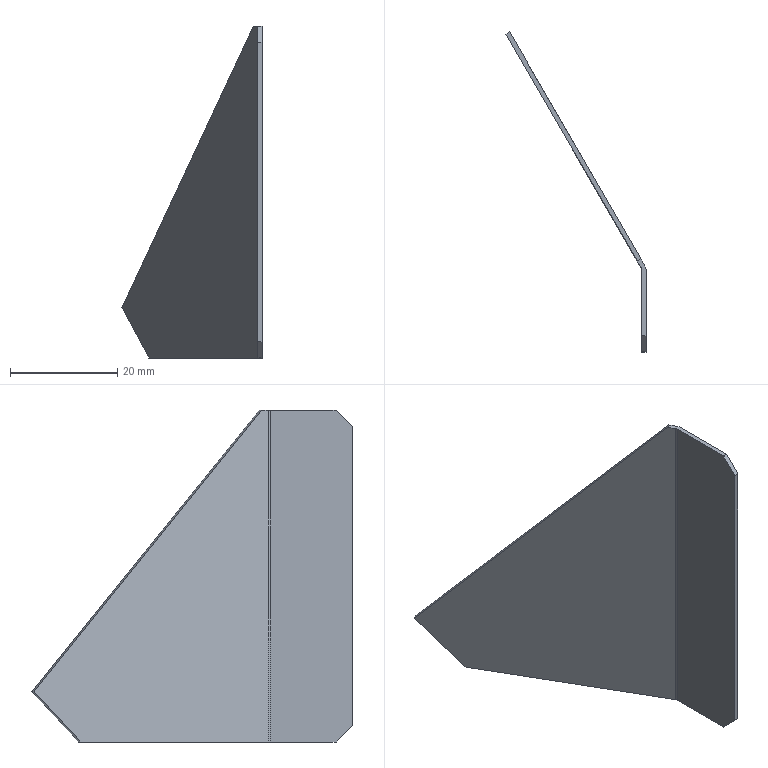Part | SolidWorks | features BaseBody 1 | 1 solid | 13 faces | box 26.168 x 59.793 x 62 mm | volume 2216 mm3 | plane 11 | cylinder 2 | commonest cylinder face diameters 1.473 x1 3.073 x1
STEP:
#1=CARTESIAN_POINT('',(267.101,174.773,-56.848));
#2=VERTEX_POINT('',#1);
#3=CARTESIAN_POINT('',(246.859,209.834,-56.848));
#4=VERTEX_POINT('',#3);
#5=CARTESIAN_POINT('',(256.98,192.304,-56.848));
#6=DIRECTION('',(-0.5,0.866,0.));
#7=VECTOR('',#6,1000.);
#8=LINE('',#5,#7);
#9=EDGE_CURVE('',#2,#4,#8,.T.);
#10=ORIENTED_EDGE('',*,*,#9,.T.);
#11=CARTESIAN_POINT('',(247.552,210.234,-56.848));
#12=VERTEX_POINT('',#11);
#13=CARTESIAN_POINT('',(247.205,210.034,-56.848));
#14=DIRECTION('',(-0.866,-0.5,0.));
#15=VECTOR('',#14,1000.);
#16=LINE('',#13,#15);
#17=EDGE_CURVE('',#12,#4,#16,.T.);
#18=ORIENTED_EDGE('',*,*,#17,.F.);
#19=CARTESIAN_POINT('',(267.794,175.173,-56.848));
#20=VERTEX_POINT('',#19);
#21=CARTESIAN_POINT('',(257.673,192.704,-56.848));
#22=DIRECTION('',(0.5,-0.866,0.));
#23=VECTOR('',#22,1000.);
#24=LINE('',#21,#23);
#25=EDGE_CURVE('',#12,#20,#24,.T.);
#26=ORIENTED_EDGE('',*,*,#25,.T.);
#27=CARTESIAN_POINT('',(268.,174.405,-56.848));
#28=VERTEX_POINT('',#27);
#29=CARTESIAN_POINT('',(266.463,174.405,-56.848));
#30=DIRECTION('',(0.,0.,-1.));
#31=DIRECTION('',(-1.,0.,0.));
#32=AXIS2_PLACEMENT_3D('',#29,#30,#31);
#33=CIRCLE('',#32,1.537);
#34=EDGE_CURVE('',#20,#28,#33,.T.);
#35=ORIENTED_EDGE('',*,*,#34,.T.);
#36=CARTESIAN_POINT('',(268.,162.147,-56.848));
#37=VERTEX_POINT('',#36);
#38=CARTESIAN_POINT('',(268.,166.776,-56.848));
#39=DIRECTION('',(0.,1.,0.));
#40=VECTOR('',#39,1000.);
#41=LINE('',#38,#40);
#42=EDGE_CURVE('',#37,#28,#41,.T.);
#43=ORIENTED_EDGE('',*,*,#42,.F.);
#44=CARTESIAN_POINT('',(267.2,162.147,-56.848));
#45=VERTEX_POINT('',#44);
#46=CARTESIAN_POINT('',(267.6,162.147,-56.848));
#47=DIRECTION('',(-1.,0.,0.));
#48=VECTOR('',#47,1000.);
#49=LINE('',#46,#48);
#50=EDGE_CURVE('',#37,#45,#49,.T.);
#51=ORIENTED_EDGE('',*,*,#50,.T.);
#52=CARTESIAN_POINT('',(267.2,174.405,-56.848));
#53=VERTEX_POINT('',#52);
#54=CARTESIAN_POINT('',(267.2,166.776,-56.848));
#55=DIRECTION('',(0.,1.,0.));
#56=VECTOR('',#55,1000.);
#57=LINE('',#54,#56);
#58=EDGE_CURVE('',#45,#53,#57,.T.);
#59=ORIENTED_EDGE('',*,*,#58,.T.);
#60=CARTESIAN_POINT('',(266.463,174.405,-56.848));
#61=DIRECTION('',(0.,0.,-1.));
#62=DIRECTION('',(-1.,0.,0.));
#63=AXIS2_PLACEMENT_3D('',#60,#61,#62);
#64=CIRCLE('',#63,0.7366);
#65=EDGE_CURVE('',#2,#53,#64,.T.);
#66=ORIENTED_EDGE('',*,*,#65,.F.);
#67=EDGE_LOOP('',(#10,#18,#26,#35,#43,#51,#59,#66));
#68=FACE_OUTER_BOUND('',#67,.T.);
#69=CARTESIAN_POINT('',(267.101,174.773,-56.848));
#70=DIRECTION('',(0.,0.,-1.));
#71=DIRECTION('',(-0.5,0.866,0.));
#72=AXIS2_PLACEMENT_3D('',#69,#70,#71);
#73=PLANE('',#72);
#74=ADVANCED_FACE('',(#68),#73,.T.);
#75=CARTESIAN_POINT('',(266.35,176.075,5.152));
#76=VERTEX_POINT('',#75);
#77=CARTESIAN_POINT('',(267.101,174.773,5.152));
#78=VERTEX_POINT('',#77);
#79=CARTESIAN_POINT('',(254.467,196.657,5.152));
#80=DIRECTION('',(0.5,-0.866,0.));
#81=VECTOR('',#80,1000.);
#82=LINE('',#79,#81);
#83=EDGE_CURVE('',#76,#78,#82,.T.);
#84=ORIENTED_EDGE('',*,*,#83,.F.);
#85=CARTESIAN_POINT('',(241.832,218.54,-47.483));
#86=VERTEX_POINT('',#85);
#87=CARTESIAN_POINT('',(241.832,218.54,-47.483));
#88=DIRECTION('',(0.3408,-0.5903,0.7317));
#89=VECTOR('',#88,1000.);
#90=LINE('',#87,#89);
#91=EDGE_CURVE('',#86,#76,#90,.T.);
#92=ORIENTED_EDGE('',*,*,#91,.F.);
#93=CARTESIAN_POINT('',(246.859,209.834,-56.848));
#94=DIRECTION('',(-0.3658,0.6337,0.6816));
#95=VECTOR('',#94,1000.);
#96=LINE('',#93,#95);
#97=EDGE_CURVE('',#4,#86,#96,.T.);
#98=ORIENTED_EDGE('',*,*,#97,.F.);
#99=ORIENTED_EDGE('',*,*,#9,.F.);
#100=CARTESIAN_POINT('',(267.101,174.773,-25.848));
#101=DIRECTION('',(0.,0.,-1.));
#102=VECTOR('',#101,1000.);
#103=LINE('',#100,#102);
#104=EDGE_CURVE('',#78,#2,#103,.T.);
#105=ORIENTED_EDGE('',*,*,#104,.F.);
#106=EDGE_LOOP('',(#84,#92,#98,#99,#105));
#107=FACE_OUTER_BOUND('',#106,.T.);
#108=CARTESIAN_POINT('',(267.101,174.773,5.152));
#109=DIRECTION('',(0.866,0.5,0.));
#110=DIRECTION('',(0.,0.,-1.));
#111=AXIS2_PLACEMENT_3D('',#108,#109,#110);
#112=PLANE('',#111);
#113=ADVANCED_FACE('',(#107),#112,.F.);
#114=CARTESIAN_POINT('',(242.525,218.94,-47.483));
#115=VERTEX_POINT('',#114);
#116=CARTESIAN_POINT('',(247.552,210.234,-56.848));
#117=DIRECTION('',(-0.3658,0.6337,0.6816));
#118=VECTOR('',#117,1000.);
#119=LINE('',#116,#118);
#120=EDGE_CURVE('',#12,#115,#119,.T.);
#121=ORIENTED_EDGE('',*,*,#120,.T.);
#122=CARTESIAN_POINT('',(267.043,176.475,5.152));
#123=VERTEX_POINT('',#122);
#124=CARTESIAN_POINT('',(242.525,218.94,-47.483));
#125=DIRECTION('',(0.3408,-0.5903,0.7317));
#126=VECTOR('',#125,1000.);
#127=LINE('',#124,#126);
#128=EDGE_CURVE('',#115,#123,#127,.T.);
#129=ORIENTED_EDGE('',*,*,#128,.T.);
#130=CARTESIAN_POINT('',(267.794,175.173,5.152));
#131=VERTEX_POINT('',#130);
#132=CARTESIAN_POINT('',(255.16,197.057,5.152));
#133=DIRECTION('',(0.5,-0.866,0.));
#134=VECTOR('',#133,1000.);
#135=LINE('',#132,#134);
#136=EDGE_CURVE('',#123,#131,#135,.T.);
#137=ORIENTED_EDGE('',*,*,#136,.T.);
#138=CARTESIAN_POINT('',(267.794,175.173,-25.848));
#139=DIRECTION('',(0.,0.,-1.));
#140=VECTOR('',#139,1000.);
#141=LINE('',#138,#140);
#142=EDGE_CURVE('',#131,#20,#141,.T.);
#143=ORIENTED_EDGE('',*,*,#142,.T.);
#144=ORIENTED_EDGE('',*,*,#25,.F.);
#145=EDGE_LOOP('',(#121,#129,#137,#143,#144));
#146=FACE_OUTER_BOUND('',#145,.T.);
#147=CARTESIAN_POINT('',(267.794,175.173,5.152));
#148=DIRECTION('',(0.866,0.5,0.));
#149=DIRECTION('',(0.,0.,-1.));
#150=AXIS2_PLACEMENT_3D('',#147,#148,#149);
#151=PLANE('',#150);
#152=ADVANCED_FACE('',(#146),#151,.T.);
#153=CARTESIAN_POINT('',(267.2,174.405,5.152));
#154=VERTEX_POINT('',#153);
#155=CARTESIAN_POINT('',(266.463,174.405,5.152));
#156=DIRECTION('',(0.,0.,1.));
#157=DIRECTION('',(-1.,0.,0.));
#158=AXIS2_PLACEMENT_3D('',#155,#156,#157);
#159=CIRCLE('',#158,0.7366);
#160=EDGE_CURVE('',#154,#78,#159,.T.);
#161=ORIENTED_EDGE('',*,*,#160,.T.);
#162=ORIENTED_EDGE('',*,*,#104,.T.);
#163=ORIENTED_EDGE('',*,*,#65,.T.);
#164=CARTESIAN_POINT('',(267.2,174.405,-25.848));
#165=DIRECTION('',(0.,0.,1.));
#166=VECTOR('',#165,1000.);
#167=LINE('',#164,#166);
#168=EDGE_CURVE('',#53,#154,#167,.T.);
#169=ORIENTED_EDGE('',*,*,#168,.T.);
#170=EDGE_LOOP('',(#161,#162,#163,#169));
#171=FACE_OUTER_BOUND('',#170,.T.);
#172=CARTESIAN_POINT('',(266.463,174.405,5.152));
#173=DIRECTION('',(0.,0.,-1.));
#174=DIRECTION('',(-1.,0.,0.));
#175=AXIS2_PLACEMENT_3D('',#172,#173,#174);
#176=CYLINDRICAL_SURFACE('',#175,0.7366);
#177=ADVANCED_FACE('',(#171),#176,.F.);
#178=ORIENTED_EDGE('',*,*,#136,.F.);
#179=CARTESIAN_POINT('',(266.696,176.275,5.152));
#180=DIRECTION('',(-0.866,-0.5,0.));
#181=VECTOR('',#180,1000.);
#182=LINE('',#179,#181);
#183=EDGE_CURVE('',#123,#76,#182,.T.);
#184=ORIENTED_EDGE('',*,*,#183,.T.);
#185=ORIENTED_EDGE('',*,*,#83,.T.);
#186=ORIENTED_EDGE('',*,*,#160,.F.);
#187=CARTESIAN_POINT('',(267.2,162.147,5.152));
#188=VERTEX_POINT('',#187);
#189=CARTESIAN_POINT('',(267.2,166.776,5.152));
#190=DIRECTION('',(0.,-1.,0.));
#191=VECTOR('',#190,1000.);
#192=LINE('',#189,#191);
#193=EDGE_CURVE('',#154,#188,#192,.T.);
#194=ORIENTED_EDGE('',*,*,#193,.T.);
#195=CARTESIAN_POINT('',(268.,162.147,5.152));
#196=VERTEX_POINT('',#195);
#197=CARTESIAN_POINT('',(267.6,162.147,5.152));
#198=DIRECTION('',(1.,0.,0.));
#199=VECTOR('',#198,1000.);
#200=LINE('',#197,#199);
#201=EDGE_CURVE('',#188,#196,#200,.T.);
#202=ORIENTED_EDGE('',*,*,#201,.T.);
#203=CARTESIAN_POINT('',(268.,174.405,5.152));
#204=VERTEX_POINT('',#203);
#205=CARTESIAN_POINT('',(268.,166.776,5.152));
#206=DIRECTION('',(0.,-1.,0.));
#207=VECTOR('',#206,1000.);
#208=LINE('',#205,#207);
#209=EDGE_CURVE('',#204,#196,#208,.T.);
#210=ORIENTED_EDGE('',*,*,#209,.F.);
#211=CARTESIAN_POINT('',(266.463,174.405,5.152));
#212=DIRECTION('',(0.,0.,1.));
#213=DIRECTION('',(-1.,0.,0.));
#214=AXIS2_PLACEMENT_3D('',#211,#212,#213);
#215=CIRCLE('',#214,1.537);
#216=EDGE_CURVE('',#204,#131,#215,.T.);
#217=ORIENTED_EDGE('',*,*,#216,.T.);
#218=EDGE_LOOP('',(#178,#184,#185,#186,#194,#202,#210,#217));
#219=FACE_OUTER_BOUND('',#218,.T.);
#220=CARTESIAN_POINT('',(266.35,176.075,5.152));
#221=DIRECTION('',(0.,0.,1.));
#222=DIRECTION('',(0.5,-0.866,0.));
#223=AXIS2_PLACEMENT_3D('',#220,#221,#222);
#224=PLANE('',#223);
#225=ADVANCED_FACE('',(#219),#224,.T.);
#226=ORIENTED_EDGE('',*,*,#91,.T.);
#227=ORIENTED_EDGE('',*,*,#183,.F.);
#228=ORIENTED_EDGE('',*,*,#128,.F.);
#229=CARTESIAN_POINT('',(242.179,218.74,-47.483));
#230=DIRECTION('',(-0.866,-0.5,0.));
#231=VECTOR('',#230,1000.);
#232=LINE('',#229,#231);
#233=EDGE_CURVE('',#115,#86,#232,.T.);
#234=ORIENTED_EDGE('',*,*,#233,.T.);
#235=EDGE_LOOP('',(#226,#227,#228,#234));
#236=FACE_OUTER_BOUND('',#235,.T.);
#237=CARTESIAN_POINT('',(241.832,218.54,-47.483));
#238=DIRECTION('',(-0.3658,0.6337,0.6816));
#239=DIRECTION('',(0.3408,-0.5903,0.7317));
#240=AXIS2_PLACEMENT_3D('',#237,#238,#239);
#241=PLANE('',#240);
#242=ADVANCED_FACE('',(#236),#241,.T.);
#243=ORIENTED_EDGE('',*,*,#97,.T.);
#244=ORIENTED_EDGE('',*,*,#233,.F.);
#245=ORIENTED_EDGE('',*,*,#120,.F.);
#246=ORIENTED_EDGE('',*,*,#17,.T.);
#247=EDGE_LOOP('',(#243,#244,#245,#246));
#248=FACE_OUTER_BOUND('',#247,.T.);
#249=CARTESIAN_POINT('',(246.859,209.834,-56.848));
#250=DIRECTION('',(-0.3408,0.5903,-0.7317));
#251=DIRECTION('',(-0.3658,0.6337,0.6816));
#252=AXIS2_PLACEMENT_3D('',#249,#250,#251);
#253=PLANE('',#252);
#254=ADVANCED_FACE('',(#248),#253,.T.);
#255=ORIENTED_EDGE('',*,*,#142,.F.);
#256=ORIENTED_EDGE('',*,*,#216,.F.);
#257=CARTESIAN_POINT('',(268.,174.405,-25.848));
#258=DIRECTION('',(0.,0.,1.));
#259=VECTOR('',#258,1000.);
#260=LINE('',#257,#259);
#261=EDGE_CURVE('',#28,#204,#260,.T.);
#262=ORIENTED_EDGE('',*,*,#261,.F.);
#263=ORIENTED_EDGE('',*,*,#34,.F.);
#264=EDGE_LOOP('',(#255,#256,#262,#263));
#265=FACE_OUTER_BOUND('',#264,.T.);
#266=CARTESIAN_POINT('',(266.463,174.405,5.152));
#267=DIRECTION('',(0.,0.,-1.));
#268=DIRECTION('',(-1.,0.,0.));
#269=AXIS2_PLACEMENT_3D('',#266,#267,#268);
#270=CYLINDRICAL_SURFACE('',#269,1.537);
#271=ADVANCED_FACE('',(#265),#270,.T.);
#272=ORIENTED_EDGE('',*,*,#168,.F.);
#273=ORIENTED_EDGE('',*,*,#58,.F.);
#274=CARTESIAN_POINT('',(267.2,159.147,-53.848));
#275=VERTEX_POINT('',#274);
#276=CARTESIAN_POINT('',(267.2,159.147,-53.848));
#277=DIRECTION('',(0.,0.7071,-0.7071));
#278=VECTOR('',#277,1000.);
#279=LINE('',#276,#278);
#280=EDGE_CURVE('',#275,#45,#279,.T.);
#281=ORIENTED_EDGE('',*,*,#280,.F.);
#282=CARTESIAN_POINT('',(267.2,159.147,2.152));
#283=VERTEX_POINT('',#282);
#284=CARTESIAN_POINT('',(267.2,159.147,-25.848));
#285=DIRECTION('',(0.,0.,-1.));
#286=VECTOR('',#285,1000.);
#287=LINE('',#284,#286);
#288=EDGE_CURVE('',#283,#275,#287,.T.);
#289=ORIENTED_EDGE('',*,*,#288,.F.);
#290=CARTESIAN_POINT('',(267.2,162.147,5.152));
#291=DIRECTION('',(0.,-0.7071,-0.7071));
#292=VECTOR('',#291,1000.);
#293=LINE('',#290,#292);
#294=EDGE_CURVE('',#188,#283,#293,.T.);
#295=ORIENTED_EDGE('',*,*,#294,.F.);
#296=ORIENTED_EDGE('',*,*,#193,.F.);
#297=EDGE_LOOP('',(#272,#273,#281,#289,#295,#296));
#298=FACE_OUTER_BOUND('',#297,.T.);
#299=CARTESIAN_POINT('',(267.2,159.147,5.152));
#300=DIRECTION('',(1.,0.,0.));
#301=DIRECTION('',(0.,0.,-1.));
#302=AXIS2_PLACEMENT_3D('',#299,#300,#301);
#303=PLANE('',#302);
#304=ADVANCED_FACE('',(#298),#303,.F.);
#305=CARTESIAN_POINT('',(268.,159.147,-53.848));
#306=VERTEX_POINT('',#305);
#307=CARTESIAN_POINT('',(268.,159.147,-53.848));
#308=DIRECTION('',(0.,0.7071,-0.7071));
#309=VECTOR('',#308,1000.);
#310=LINE('',#307,#309);
#311=EDGE_CURVE('',#306,#37,#310,.T.);
#312=ORIENTED_EDGE('',*,*,#311,.T.);
#313=ORIENTED_EDGE('',*,*,#42,.T.);
#314=ORIENTED_EDGE('',*,*,#261,.T.);
#315=ORIENTED_EDGE('',*,*,#209,.T.);
#316=CARTESIAN_POINT('',(268.,159.147,2.152));
#317=VERTEX_POINT('',#316);
#318=CARTESIAN_POINT('',(268.,162.147,5.152));
#319=DIRECTION('',(0.,-0.7071,-0.7071));
#320=VECTOR('',#319,1000.);
#321=LINE('',#318,#320);
#322=EDGE_CURVE('',#196,#317,#321,.T.);
#323=ORIENTED_EDGE('',*,*,#322,.T.);
#324=CARTESIAN_POINT('',(268.,159.147,-25.848));
#325=DIRECTION('',(0.,0.,-1.));
#326=VECTOR('',#325,1000.);
#327=LINE('',#324,#326);
#328=EDGE_CURVE('',#317,#306,#327,.T.);
#329=ORIENTED_EDGE('',*,*,#328,.T.);
#330=EDGE_LOOP('',(#312,#313,#314,#315,#323,#329));
#331=FACE_OUTER_BOUND('',#330,.T.);
#332=CARTESIAN_POINT('',(268.,159.147,5.152));
#333=DIRECTION('',(1.,0.,0.));
#334=DIRECTION('',(0.,0.,-1.));
#335=AXIS2_PLACEMENT_3D('',#332,#333,#334);
#336=PLANE('',#335);
#337=ADVANCED_FACE('',(#331),#336,.T.);
#338=ORIENTED_EDGE('',*,*,#280,.T.);
#339=ORIENTED_EDGE('',*,*,#50,.F.);
#340=ORIENTED_EDGE('',*,*,#311,.F.);
#341=CARTESIAN_POINT('',(267.6,159.147,-53.848));
#342=DIRECTION('',(-1.,0.,0.));
#343=VECTOR('',#342,1000.);
#344=LINE('',#341,#343);
#345=EDGE_CURVE('',#306,#275,#344,.T.);
#346=ORIENTED_EDGE('',*,*,#345,.T.);
#347=EDGE_LOOP('',(#338,#339,#340,#346));
#348=FACE_OUTER_BOUND('',#347,.T.);
#349=CARTESIAN_POINT('',(267.2,159.147,-53.848));
#350=DIRECTION('',(0.,-0.7071,-0.7071));
#351=DIRECTION('',(0.,0.7071,-0.7071));
#352=AXIS2_PLACEMENT_3D('',#349,#350,#351);
#353=PLANE('',#352);
#354=ADVANCED_FACE('',(#348),#353,.T.);
#355=ORIENTED_EDGE('',*,*,#288,.T.);
#356=ORIENTED_EDGE('',*,*,#345,.F.);
#357=ORIENTED_EDGE('',*,*,#328,.F.);
#358=CARTESIAN_POINT('',(267.6,159.147,2.152));
#359=DIRECTION('',(-1.,0.,0.));
#360=VECTOR('',#359,1000.);
#361=LINE('',#358,#360);
#362=EDGE_CURVE('',#317,#283,#361,.T.);
#363=ORIENTED_EDGE('',*,*,#362,.T.);
#364=EDGE_LOOP('',(#355,#356,#357,#363));
#365=FACE_OUTER_BOUND('',#364,.T.);
#366=CARTESIAN_POINT('',(267.2,159.147,2.152));
#367=DIRECTION('',(0.,-1.,0.));
#368=DIRECTION('',(0.,0.,-1.));
#369=AXIS2_PLACEMENT_3D('',#366,#367,#368);
#370=PLANE('',#369);
#371=ADVANCED_FACE('',(#365),#370,.T.);
#372=ORIENTED_EDGE('',*,*,#294,.T.);
#373=ORIENTED_EDGE('',*,*,#362,.F.);
#374=ORIENTED_EDGE('',*,*,#322,.F.);
#375=ORIENTED_EDGE('',*,*,#201,.F.);
#376=EDGE_LOOP('',(#372,#373,#374,#375));
#377=FACE_OUTER_BOUND('',#376,.T.);
#378=CARTESIAN_POINT('',(267.2,162.147,5.152));
#379=DIRECTION('',(0.,-0.7071,0.7071));
#380=DIRECTION('',(0.,-0.7071,-0.7071));
#381=AXIS2_PLACEMENT_3D('',#378,#379,#380);
#382=PLANE('',#381);
#383=ADVANCED_FACE('',(#377),#382,.T.);
#384=CLOSED_SHELL('',(#74,#113,#152,#177,#225,#242,#254,#271,#304,#337,#354,#371,#383));
#385=MANIFOLD_SOLID_BREP('',#384);
#386=CARTESIAN_POINT('',(0.,0.,0.));
#387=DIRECTION('',(0.,0.,1.));
#388=DIRECTION('',(1.,0.,0.));
#389=AXIS2_PLACEMENT_3D('',#386,#387,#388);
#390=(LENGTH_UNIT()NAMED_UNIT(*)SI_UNIT(.MILLI.,.METRE.));
#391=UNCERTAINTY_MEASURE_WITH_UNIT(LENGTH_MEASURE(0.00001),#390,'','');
#392=(NAMED_UNIT(*)PLANE_ANGLE_UNIT()SI_UNIT($,.RADIAN.));
#393=(NAMED_UNIT(*)SI_UNIT($,.STERADIAN.)SOLID_ANGLE_UNIT());
#394=(GEOMETRIC_REPRESENTATION_CONTEXT(3)GLOBAL_UNCERTAINTY_ASSIGNED_CONTEXT((#391))GLOBAL_UNIT_ASSIGNED_CONTEXT((#390,#392,#393))REPRESENTATION_CONTEXT('',''));
#395=ADVANCED_BREP_SHAPE_REPRESENTATION('',(#385,#389),#394);